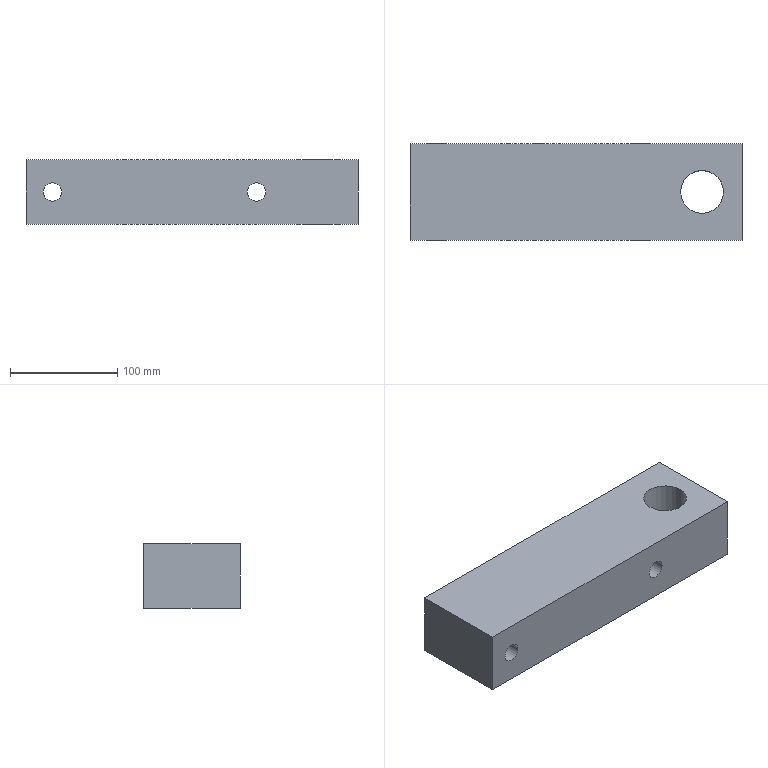Part | SolidWorks | features ICE 2, Extrusion 1, HoleWzd 1 | 1 solid | 16 faces | box 310 x 90 x 60 mm | volume 1555190 mm3 | cylinder 8 | plane 6 | cone 2 | commonest cylinder face diameters 17 x4 10.2 x2 40 x2
STEP:
#1=CARTESIAN_POINT('',(137.7,0.,60.));
#2=VERTEX_POINT('',#1);
#3=CARTESIAN_POINT('',(97.7,0.,60.));
#4=VERTEX_POINT('',#3);
#5=CARTESIAN_POINT('',(117.7,0.,60.));
#6=DIRECTION('',(0.,0.,-1.));
#7=DIRECTION('',(-1.,0.,0.));
#8=AXIS2_PLACEMENT_3D('',#5,#6,#7);
#9=CIRCLE('',#8,20.);
#10=EDGE_CURVE('',#2,#4,#9,.T.);
#11=ORIENTED_EDGE('',*,*,#10,.F.);
#12=CARTESIAN_POINT('',(137.7,0.,0.));
#13=VERTEX_POINT('',#12);
#14=CARTESIAN_POINT('',(137.7,0.,60.));
#15=DIRECTION('',(0.,0.,-1.));
#16=VECTOR('',#15,1000.);
#17=LINE('',#14,#16);
#18=EDGE_CURVE('',#2,#13,#17,.T.);
#19=ORIENTED_EDGE('',*,*,#18,.T.);
#20=CARTESIAN_POINT('',(97.7,0.,0.));
#21=VERTEX_POINT('',#20);
#22=CARTESIAN_POINT('',(117.7,0.,0.));
#23=DIRECTION('',(0.,0.,-1.));
#24=DIRECTION('',(-1.,0.,0.));
#25=AXIS2_PLACEMENT_3D('',#22,#23,#24);
#26=CIRCLE('',#25,20.);
#27=EDGE_CURVE('',#13,#21,#26,.T.);
#28=ORIENTED_EDGE('',*,*,#27,.T.);
#29=CARTESIAN_POINT('',(97.7,0.,60.));
#30=DIRECTION('',(0.,0.,-1.));
#31=VECTOR('',#30,1000.);
#32=LINE('',#29,#31);
#33=EDGE_CURVE('',#4,#21,#32,.T.);
#34=ORIENTED_EDGE('',*,*,#33,.F.);
#35=EDGE_LOOP('',(#11,#19,#28,#34));
#36=FACE_OUTER_BOUND('',#35,.T.);
#37=CARTESIAN_POINT('',(117.7,0.,60.));
#38=DIRECTION('',(0.,0.,-1.));
#39=DIRECTION('',(-1.,0.,0.));
#40=AXIS2_PLACEMENT_3D('',#37,#38,#39);
#41=CYLINDRICAL_SURFACE('',#40,20.);
#42=ADVANCED_FACE('',(#36),#41,.F.);
#43=CARTESIAN_POINT('',(-35.,14.75,24.9));
#44=VERTEX_POINT('',#43);
#45=CARTESIAN_POINT('',(-35.,14.75,35.1));
#46=VERTEX_POINT('',#45);
#47=CARTESIAN_POINT('',(-35.,14.75,30.));
#48=DIRECTION('',(0.,1.,0.));
#49=DIRECTION('',(0.,0.,1.));
#50=AXIS2_PLACEMENT_3D('',#47,#48,#49);
#51=CIRCLE('',#50,5.1);
#52=EDGE_CURVE('',#44,#46,#51,.T.);
#53=ORIENTED_EDGE('',*,*,#52,.F.);
#54=CARTESIAN_POINT('',(-35.,45.,24.9));
#55=VERTEX_POINT('',#54);
#56=CARTESIAN_POINT('',(-35.,45.,24.9));
#57=DIRECTION('',(0.,1.,0.));
#58=VECTOR('',#57,1000.);
#59=LINE('',#56,#58);
#60=EDGE_CURVE('',#44,#55,#59,.T.);
#61=ORIENTED_EDGE('',*,*,#60,.T.);
#62=CARTESIAN_POINT('',(-35.,45.,35.1));
#63=VERTEX_POINT('',#62);
#64=CARTESIAN_POINT('',(-35.,45.,30.));
#65=DIRECTION('',(0.,1.,0.));
#66=DIRECTION('',(0.,0.,1.));
#67=AXIS2_PLACEMENT_3D('',#64,#65,#66);
#68=CIRCLE('',#67,5.1);
#69=EDGE_CURVE('',#55,#63,#68,.T.);
#70=ORIENTED_EDGE('',*,*,#69,.T.);
#71=CARTESIAN_POINT('',(-35.,45.,35.1));
#72=DIRECTION('',(0.,1.,0.));
#73=VECTOR('',#72,1000.);
#74=LINE('',#71,#73);
#75=EDGE_CURVE('',#46,#63,#74,.T.);
#76=ORIENTED_EDGE('',*,*,#75,.F.);
#77=EDGE_LOOP('',(#53,#61,#70,#76));
#78=FACE_OUTER_BOUND('',#77,.T.);
#79=CARTESIAN_POINT('',(-35.,45.,30.));
#80=DIRECTION('',(0.,1.,0.));
#81=DIRECTION('',(0.,0.,1.));
#82=AXIS2_PLACEMENT_3D('',#79,#80,#81);
#83=CYLINDRICAL_SURFACE('',#82,5.1);
#84=ADVANCED_FACE('',(#78),#83,.F.);
#85=CARTESIAN_POINT('',(-35.,11.686,30.));
#86=VERTEX_POINT('',#85);
#87=CARTESIAN_POINT('',(-35.,14.75,35.1));
#88=DIRECTION('',(0.,0.515,0.8572));
#89=VECTOR('',#88,1000.);
#90=LINE('',#87,#89);
#91=EDGE_CURVE('',#86,#46,#90,.T.);
#92=ORIENTED_EDGE('',*,*,#91,.F.);
#93=CARTESIAN_POINT('',(-35.,14.75,24.9));
#94=DIRECTION('',(0.,0.515,-0.8572));
#95=VECTOR('',#94,1000.);
#96=LINE('',#93,#95);
#97=EDGE_CURVE('',#86,#44,#96,.T.);
#98=ORIENTED_EDGE('',*,*,#97,.T.);
#99=ORIENTED_EDGE('',*,*,#52,.T.);
#100=EDGE_LOOP('',(#92,#98,#99));
#101=FACE_OUTER_BOUND('',#100,.T.);
#102=CARTESIAN_POINT('',(-35.,14.75,30.));
#103=DIRECTION('',(0.,1.,0.));
#104=DIRECTION('',(0.,0.,1.));
#105=AXIS2_PLACEMENT_3D('',#102,#103,#104);
#106=CONICAL_SURFACE('',#105,5.1,1.03);
#107=ADVANCED_FACE('',(#101),#106,.F.);
#108=CARTESIAN_POINT('',(-121.75,-45.,30.));
#109=VERTEX_POINT('',#108);
#110=CARTESIAN_POINT('',(-138.75,-45.,30.));
#111=VERTEX_POINT('',#110);
#112=CARTESIAN_POINT('',(-130.25,-45.,30.));
#113=DIRECTION('',(0.,1.,0.));
#114=DIRECTION('',(-1.,0.,0.));
#115=AXIS2_PLACEMENT_3D('',#112,#113,#114);
#116=CIRCLE('',#115,8.5);
#117=EDGE_CURVE('',#109,#111,#116,.T.);
#118=ORIENTED_EDGE('',*,*,#117,.F.);
#119=CARTESIAN_POINT('',(-121.75,45.,30.));
#120=VERTEX_POINT('',#119);
#121=CARTESIAN_POINT('',(-121.75,-45.,30.));
#122=DIRECTION('',(0.,1.,0.));
#123=VECTOR('',#122,1000.);
#124=LINE('',#121,#123);
#125=EDGE_CURVE('',#109,#120,#124,.T.);
#126=ORIENTED_EDGE('',*,*,#125,.T.);
#127=CARTESIAN_POINT('',(-138.75,45.,30.));
#128=VERTEX_POINT('',#127);
#129=CARTESIAN_POINT('',(-130.25,45.,30.));
#130=DIRECTION('',(0.,1.,0.));
#131=DIRECTION('',(-1.,0.,0.));
#132=AXIS2_PLACEMENT_3D('',#129,#130,#131);
#133=CIRCLE('',#132,8.5);
#134=EDGE_CURVE('',#120,#128,#133,.T.);
#135=ORIENTED_EDGE('',*,*,#134,.T.);
#136=CARTESIAN_POINT('',(-138.75,-45.,30.));
#137=DIRECTION('',(0.,1.,0.));
#138=VECTOR('',#137,1000.);
#139=LINE('',#136,#138);
#140=EDGE_CURVE('',#111,#128,#139,.T.);
#141=ORIENTED_EDGE('',*,*,#140,.F.);
#142=EDGE_LOOP('',(#118,#126,#135,#141));
#143=FACE_OUTER_BOUND('',#142,.T.);
#144=CARTESIAN_POINT('',(-130.25,-45.,30.));
#145=DIRECTION('',(0.,1.,0.));
#146=DIRECTION('',(-1.,0.,0.));
#147=AXIS2_PLACEMENT_3D('',#144,#145,#146);
#148=CYLINDRICAL_SURFACE('',#147,8.5);
#149=ADVANCED_FACE('',(#143),#148,.F.);
#150=CARTESIAN_POINT('',(68.75,-45.,30.));
#151=VERTEX_POINT('',#150);
#152=CARTESIAN_POINT('',(51.75,-45.,30.));
#153=VERTEX_POINT('',#152);
#154=CARTESIAN_POINT('',(60.25,-45.,30.));
#155=DIRECTION('',(0.,1.,0.));
#156=DIRECTION('',(-1.,0.,0.));
#157=AXIS2_PLACEMENT_3D('',#154,#155,#156);
#158=CIRCLE('',#157,8.5);
#159=EDGE_CURVE('',#151,#153,#158,.T.);
#160=ORIENTED_EDGE('',*,*,#159,.F.);
#161=CARTESIAN_POINT('',(68.75,45.,30.));
#162=VERTEX_POINT('',#161);
#163=CARTESIAN_POINT('',(68.75,-45.,30.));
#164=DIRECTION('',(0.,1.,0.));
#165=VECTOR('',#164,1000.);
#166=LINE('',#163,#165);
#167=EDGE_CURVE('',#151,#162,#166,.T.);
#168=ORIENTED_EDGE('',*,*,#167,.T.);
#169=CARTESIAN_POINT('',(51.75,45.,30.));
#170=VERTEX_POINT('',#169);
#171=CARTESIAN_POINT('',(60.25,45.,30.));
#172=DIRECTION('',(0.,1.,0.));
#173=DIRECTION('',(-1.,0.,0.));
#174=AXIS2_PLACEMENT_3D('',#171,#172,#173);
#175=CIRCLE('',#174,8.5);
#176=EDGE_CURVE('',#162,#170,#175,.T.);
#177=ORIENTED_EDGE('',*,*,#176,.T.);
#178=CARTESIAN_POINT('',(51.75,-45.,30.));
#179=DIRECTION('',(0.,1.,0.));
#180=VECTOR('',#179,1000.);
#181=LINE('',#178,#180);
#182=EDGE_CURVE('',#153,#170,#181,.T.);
#183=ORIENTED_EDGE('',*,*,#182,.F.);
#184=EDGE_LOOP('',(#160,#168,#177,#183));
#185=FACE_OUTER_BOUND('',#184,.T.);
#186=CARTESIAN_POINT('',(60.25,-45.,30.));
#187=DIRECTION('',(0.,1.,0.));
#188=DIRECTION('',(-1.,0.,0.));
#189=AXIS2_PLACEMENT_3D('',#186,#187,#188);
#190=CYLINDRICAL_SURFACE('',#189,8.5);
#191=ADVANCED_FACE('',(#185),#190,.F.);
#192=CARTESIAN_POINT('',(-155.,45.,0.));
#193=VERTEX_POINT('',#192);
#194=CARTESIAN_POINT('',(-155.,-45.,0.));
#195=VERTEX_POINT('',#194);
#196=CARTESIAN_POINT('',(-155.,45.,0.));
#197=DIRECTION('',(0.,-1.,0.));
#198=VECTOR('',#197,1000.);
#199=LINE('',#196,#198);
#200=EDGE_CURVE('',#193,#195,#199,.T.);
#201=ORIENTED_EDGE('',*,*,#200,.T.);
#202=CARTESIAN_POINT('',(-155.,-45.,60.));
#203=VERTEX_POINT('',#202);
#204=CARTESIAN_POINT('',(-155.,-45.,60.));
#205=DIRECTION('',(0.,0.,-1.));
#206=VECTOR('',#205,1000.);
#207=LINE('',#204,#206);
#208=EDGE_CURVE('',#203,#195,#207,.T.);
#209=ORIENTED_EDGE('',*,*,#208,.F.);
#210=CARTESIAN_POINT('',(-155.,45.,60.));
#211=VERTEX_POINT('',#210);
#212=CARTESIAN_POINT('',(-155.,45.,60.));
#213=DIRECTION('',(0.,-1.,0.));
#214=VECTOR('',#213,1000.);
#215=LINE('',#212,#214);
#216=EDGE_CURVE('',#211,#203,#215,.T.);
#217=ORIENTED_EDGE('',*,*,#216,.F.);
#218=CARTESIAN_POINT('',(-155.,45.,60.));
#219=DIRECTION('',(0.,0.,-1.));
#220=VECTOR('',#219,1000.);
#221=LINE('',#218,#220);
#222=EDGE_CURVE('',#211,#193,#221,.T.);
#223=ORIENTED_EDGE('',*,*,#222,.T.);
#224=EDGE_LOOP('',(#201,#209,#217,#223));
#225=FACE_OUTER_BOUND('',#224,.T.);
#226=CARTESIAN_POINT('',(-155.,45.,60.));
#227=DIRECTION('',(1.,0.,0.));
#228=DIRECTION('',(0.,0.,-1.));
#229=AXIS2_PLACEMENT_3D('',#226,#227,#228);
#230=PLANE('',#229);
#231=ADVANCED_FACE('',(#225),#230,.F.);
#232=CARTESIAN_POINT('',(-130.25,-45.,30.));
#233=DIRECTION('',(0.,1.,0.));
#234=DIRECTION('',(-1.,0.,0.));
#235=AXIS2_PLACEMENT_3D('',#232,#233,#234);
#236=CIRCLE('',#235,8.5);
#237=EDGE_CURVE('',#111,#109,#236,.T.);
#238=ORIENTED_EDGE('',*,*,#237,.T.);
#239=ORIENTED_EDGE('',*,*,#117,.T.);
#240=EDGE_LOOP('',(#238,#239));
#241=FACE_BOUND('',#240,.T.);
#242=CARTESIAN_POINT('',(60.25,-45.,30.));
#243=DIRECTION('',(0.,1.,0.));
#244=DIRECTION('',(-1.,0.,0.));
#245=AXIS2_PLACEMENT_3D('',#242,#243,#244);
#246=CIRCLE('',#245,8.5);
#247=EDGE_CURVE('',#153,#151,#246,.T.);
#248=ORIENTED_EDGE('',*,*,#247,.T.);
#249=ORIENTED_EDGE('',*,*,#159,.T.);
#250=EDGE_LOOP('',(#248,#249));
#251=FACE_BOUND('',#250,.T.);
#252=CARTESIAN_POINT('',(155.,-45.,0.));
#253=VERTEX_POINT('',#252);
#254=CARTESIAN_POINT('',(155.,-45.,0.));
#255=DIRECTION('',(1.,0.,0.));
#256=VECTOR('',#255,1000.);
#257=LINE('',#254,#256);
#258=EDGE_CURVE('',#195,#253,#257,.T.);
#259=ORIENTED_EDGE('',*,*,#258,.T.);
#260=CARTESIAN_POINT('',(155.,-45.,60.));
#261=VERTEX_POINT('',#260);
#262=CARTESIAN_POINT('',(155.,-45.,60.));
#263=DIRECTION('',(0.,0.,-1.));
#264=VECTOR('',#263,1000.);
#265=LINE('',#262,#264);
#266=EDGE_CURVE('',#261,#253,#265,.T.);
#267=ORIENTED_EDGE('',*,*,#266,.F.);
#268=CARTESIAN_POINT('',(155.,-45.,60.));
#269=DIRECTION('',(1.,0.,0.));
#270=VECTOR('',#269,1000.);
#271=LINE('',#268,#270);
#272=EDGE_CURVE('',#203,#261,#271,.T.);
#273=ORIENTED_EDGE('',*,*,#272,.F.);
#274=ORIENTED_EDGE('',*,*,#208,.T.);
#275=EDGE_LOOP('',(#259,#267,#273,#274));
#276=FACE_OUTER_BOUND('',#275,.T.);
#277=CARTESIAN_POINT('',(155.,-45.,60.));
#278=DIRECTION('',(0.,1.,0.));
#279=DIRECTION('',(-1.,0.,0.));
#280=AXIS2_PLACEMENT_3D('',#277,#278,#279);
#281=PLANE('',#280);
#282=ADVANCED_FACE('',(#241,#251,#276),#281,.F.);
#283=CARTESIAN_POINT('',(155.,45.,0.));
#284=VERTEX_POINT('',#283);
#285=CARTESIAN_POINT('',(155.,45.,0.));
#286=DIRECTION('',(0.,1.,0.));
#287=VECTOR('',#286,1000.);
#288=LINE('',#285,#287);
#289=EDGE_CURVE('',#253,#284,#288,.T.);
#290=ORIENTED_EDGE('',*,*,#289,.T.);
#291=CARTESIAN_POINT('',(155.,45.,60.));
#292=VERTEX_POINT('',#291);
#293=CARTESIAN_POINT('',(155.,45.,60.));
#294=DIRECTION('',(0.,0.,-1.));
#295=VECTOR('',#294,1000.);
#296=LINE('',#293,#295);
#297=EDGE_CURVE('',#292,#284,#296,.T.);
#298=ORIENTED_EDGE('',*,*,#297,.F.);
#299=CARTESIAN_POINT('',(155.,45.,60.));
#300=DIRECTION('',(0.,1.,0.));
#301=VECTOR('',#300,1000.);
#302=LINE('',#299,#301);
#303=EDGE_CURVE('',#261,#292,#302,.T.);
#304=ORIENTED_EDGE('',*,*,#303,.F.);
#305=ORIENTED_EDGE('',*,*,#266,.T.);
#306=EDGE_LOOP('',(#290,#298,#304,#305));
#307=FACE_OUTER_BOUND('',#306,.T.);
#308=CARTESIAN_POINT('',(155.,45.,60.));
#309=DIRECTION('',(-1.,0.,0.));
#310=DIRECTION('',(0.,0.,1.));
#311=AXIS2_PLACEMENT_3D('',#308,#309,#310);
#312=PLANE('',#311);
#313=ADVANCED_FACE('',(#307),#312,.F.);
#314=CARTESIAN_POINT('',(-35.,45.,30.));
#315=DIRECTION('',(0.,1.,0.));
#316=DIRECTION('',(0.,0.,1.));
#317=AXIS2_PLACEMENT_3D('',#314,#315,#316);
#318=CIRCLE('',#317,5.1);
#319=EDGE_CURVE('',#63,#55,#318,.T.);
#320=ORIENTED_EDGE('',*,*,#319,.F.);
#321=ORIENTED_EDGE('',*,*,#69,.F.);
#322=EDGE_LOOP('',(#320,#321));
#323=FACE_BOUND('',#322,.T.);
#324=CARTESIAN_POINT('',(-130.25,45.,30.));
#325=DIRECTION('',(0.,1.,0.));
#326=DIRECTION('',(-1.,0.,0.));
#327=AXIS2_PLACEMENT_3D('',#324,#325,#326);
#328=CIRCLE('',#327,8.5);
#329=EDGE_CURVE('',#128,#120,#328,.T.);
#330=ORIENTED_EDGE('',*,*,#329,.F.);
#331=ORIENTED_EDGE('',*,*,#134,.F.);
#332=EDGE_LOOP('',(#330,#331));
#333=FACE_BOUND('',#332,.T.);
#334=CARTESIAN_POINT('',(60.25,45.,30.));
#335=DIRECTION('',(0.,1.,0.));
#336=DIRECTION('',(-1.,0.,0.));
#337=AXIS2_PLACEMENT_3D('',#334,#335,#336);
#338=CIRCLE('',#337,8.5);
#339=EDGE_CURVE('',#170,#162,#338,.T.);
#340=ORIENTED_EDGE('',*,*,#339,.F.);
#341=ORIENTED_EDGE('',*,*,#176,.F.);
#342=EDGE_LOOP('',(#340,#341));
#343=FACE_BOUND('',#342,.T.);
#344=CARTESIAN_POINT('',(155.,45.,0.));
#345=DIRECTION('',(-1.,0.,0.));
#346=VECTOR('',#345,1000.);
#347=LINE('',#344,#346);
#348=EDGE_CURVE('',#284,#193,#347,.T.);
#349=ORIENTED_EDGE('',*,*,#348,.T.);
#350=ORIENTED_EDGE('',*,*,#222,.F.);
#351=CARTESIAN_POINT('',(155.,45.,60.));
#352=DIRECTION('',(-1.,0.,0.));
#353=VECTOR('',#352,1000.);
#354=LINE('',#351,#353);
#355=EDGE_CURVE('',#292,#211,#354,.T.);
#356=ORIENTED_EDGE('',*,*,#355,.F.);
#357=ORIENTED_EDGE('',*,*,#297,.T.);
#358=EDGE_LOOP('',(#349,#350,#356,#357));
#359=FACE_OUTER_BOUND('',#358,.T.);
#360=CARTESIAN_POINT('',(155.,45.,60.));
#361=DIRECTION('',(0.,-1.,0.));
#362=DIRECTION('',(1.,0.,0.));
#363=AXIS2_PLACEMENT_3D('',#360,#361,#362);
#364=PLANE('',#363);
#365=ADVANCED_FACE('',(#323,#333,#343,#359),#364,.F.);
#366=CARTESIAN_POINT('',(117.7,0.,60.));
#367=DIRECTION('',(0.,0.,-1.));
#368=DIRECTION('',(-1.,0.,0.));
#369=AXIS2_PLACEMENT_3D('',#366,#367,#368);
#370=CIRCLE('',#369,20.);
#371=EDGE_CURVE('',#4,#2,#370,.T.);
#372=ORIENTED_EDGE('',*,*,#371,.T.);
#373=ORIENTED_EDGE('',*,*,#10,.T.);
#374=EDGE_LOOP('',(#372,#373));
#375=FACE_BOUND('',#374,.T.);
#376=ORIENTED_EDGE('',*,*,#216,.T.);
#377=ORIENTED_EDGE('',*,*,#272,.T.);
#378=ORIENTED_EDGE('',*,*,#303,.T.);
#379=ORIENTED_EDGE('',*,*,#355,.T.);
#380=EDGE_LOOP('',(#376,#377,#378,#379));
#381=FACE_OUTER_BOUND('',#380,.T.);
#382=CARTESIAN_POINT('',(0.,0.,60.));
#383=DIRECTION('',(0.,0.,-1.));
#384=DIRECTION('',(-1.,0.,0.));
#385=AXIS2_PLACEMENT_3D('',#382,#383,#384);
#386=PLANE('',#385);
#387=ADVANCED_FACE('',(#375,#381),#386,.F.);
#388=CARTESIAN_POINT('',(117.7,0.,0.));
#389=DIRECTION('',(0.,0.,-1.));
#390=DIRECTION('',(-1.,0.,0.));
#391=AXIS2_PLACEMENT_3D('',#388,#389,#390);
#392=CIRCLE('',#391,20.);
#393=EDGE_CURVE('',#21,#13,#392,.T.);
#394=ORIENTED_EDGE('',*,*,#393,.F.);
#395=ORIENTED_EDGE('',*,*,#27,.F.);
#396=EDGE_LOOP('',(#394,#395));
#397=FACE_BOUND('',#396,.T.);
#398=ORIENTED_EDGE('',*,*,#200,.F.);
#399=ORIENTED_EDGE('',*,*,#348,.F.);
#400=ORIENTED_EDGE('',*,*,#289,.F.);
#401=ORIENTED_EDGE('',*,*,#258,.F.);
#402=EDGE_LOOP('',(#398,#399,#400,#401));
#403=FACE_OUTER_BOUND('',#402,.T.);
#404=CARTESIAN_POINT('',(0.,0.,0.));
#405=DIRECTION('',(0.,0.,-1.));
#406=DIRECTION('',(-1.,0.,0.));
#407=AXIS2_PLACEMENT_3D('',#404,#405,#406);
#408=PLANE('',#407);
#409=ADVANCED_FACE('',(#397,#403),#408,.T.);
#410=ORIENTED_EDGE('',*,*,#167,.F.);
#411=ORIENTED_EDGE('',*,*,#247,.F.);
#412=ORIENTED_EDGE('',*,*,#182,.T.);
#413=ORIENTED_EDGE('',*,*,#339,.T.);
#414=EDGE_LOOP('',(#410,#411,#412,#413));
#415=FACE_OUTER_BOUND('',#414,.T.);
#416=CARTESIAN_POINT('',(60.25,-45.,30.));
#417=DIRECTION('',(0.,1.,0.));
#418=DIRECTION('',(-1.,0.,0.));
#419=AXIS2_PLACEMENT_3D('',#416,#417,#418);
#420=CYLINDRICAL_SURFACE('',#419,8.5);
#421=ADVANCED_FACE('',(#415),#420,.F.);
#422=ORIENTED_EDGE('',*,*,#125,.F.);
#423=ORIENTED_EDGE('',*,*,#237,.F.);
#424=ORIENTED_EDGE('',*,*,#140,.T.);
#425=ORIENTED_EDGE('',*,*,#329,.T.);
#426=EDGE_LOOP('',(#422,#423,#424,#425));
#427=FACE_OUTER_BOUND('',#426,.T.);
#428=CARTESIAN_POINT('',(-130.25,-45.,30.));
#429=DIRECTION('',(0.,1.,0.));
#430=DIRECTION('',(-1.,0.,0.));
#431=AXIS2_PLACEMENT_3D('',#428,#429,#430);
#432=CYLINDRICAL_SURFACE('',#431,8.5);
#433=ADVANCED_FACE('',(#427),#432,.F.);
#434=ORIENTED_EDGE('',*,*,#97,.F.);
#435=ORIENTED_EDGE('',*,*,#91,.T.);
#436=CARTESIAN_POINT('',(-35.,14.75,30.));
#437=DIRECTION('',(0.,1.,0.));
#438=DIRECTION('',(0.,0.,1.));
#439=AXIS2_PLACEMENT_3D('',#436,#437,#438);
#440=CIRCLE('',#439,5.1);
#441=EDGE_CURVE('',#46,#44,#440,.T.);
#442=ORIENTED_EDGE('',*,*,#441,.T.);
#443=EDGE_LOOP('',(#434,#435,#442));
#444=FACE_OUTER_BOUND('',#443,.T.);
#445=CARTESIAN_POINT('',(-35.,14.75,30.));
#446=DIRECTION('',(0.,1.,0.));
#447=DIRECTION('',(0.,0.,1.));
#448=AXIS2_PLACEMENT_3D('',#445,#446,#447);
#449=CONICAL_SURFACE('',#448,5.1,1.03);
#450=ADVANCED_FACE('',(#444),#449,.F.);
#451=ORIENTED_EDGE('',*,*,#60,.F.);
#452=ORIENTED_EDGE('',*,*,#441,.F.);
#453=ORIENTED_EDGE('',*,*,#75,.T.);
#454=ORIENTED_EDGE('',*,*,#319,.T.);
#455=EDGE_LOOP('',(#451,#452,#453,#454));
#456=FACE_OUTER_BOUND('',#455,.T.);
#457=CARTESIAN_POINT('',(-35.,45.,30.));
#458=DIRECTION('',(0.,1.,0.));
#459=DIRECTION('',(0.,0.,1.));
#460=AXIS2_PLACEMENT_3D('',#457,#458,#459);
#461=CYLINDRICAL_SURFACE('',#460,5.1);
#462=ADVANCED_FACE('',(#456),#461,.F.);
#463=ORIENTED_EDGE('',*,*,#18,.F.);
#464=ORIENTED_EDGE('',*,*,#371,.F.);
#465=ORIENTED_EDGE('',*,*,#33,.T.);
#466=ORIENTED_EDGE('',*,*,#393,.T.);
#467=EDGE_LOOP('',(#463,#464,#465,#466));
#468=FACE_OUTER_BOUND('',#467,.T.);
#469=CARTESIAN_POINT('',(117.7,0.,60.));
#470=DIRECTION('',(0.,0.,-1.));
#471=DIRECTION('',(-1.,0.,0.));
#472=AXIS2_PLACEMENT_3D('',#469,#470,#471);
#473=CYLINDRICAL_SURFACE('',#472,20.);
#474=ADVANCED_FACE('',(#468),#473,.F.);
#475=CLOSED_SHELL('',(#42,#84,#107,#149,#191,#231,#282,#313,#365,#387,#409,#421,#433,#450,#462,#474));
#476=MANIFOLD_SOLID_BREP('',#475);
#477=CARTESIAN_POINT('',(0.,0.,0.));
#478=DIRECTION('',(0.,0.,1.));
#479=DIRECTION('',(1.,0.,0.));
#480=AXIS2_PLACEMENT_3D('',#477,#478,#479);
#481=(LENGTH_UNIT()NAMED_UNIT(*)SI_UNIT(.MILLI.,.METRE.));
#482=UNCERTAINTY_MEASURE_WITH_UNIT(LENGTH_MEASURE(0.00001),#481,'','');
#483=(NAMED_UNIT(*)PLANE_ANGLE_UNIT()SI_UNIT($,.RADIAN.));
#484=(NAMED_UNIT(*)SI_UNIT($,.STERADIAN.)SOLID_ANGLE_UNIT());
#485=(GEOMETRIC_REPRESENTATION_CONTEXT(3)GLOBAL_UNCERTAINTY_ASSIGNED_CONTEXT((#482))GLOBAL_UNIT_ASSIGNED_CONTEXT((#481,#483,#484))REPRESENTATION_CONTEXT('',''));
#486=ADVANCED_BREP_SHAPE_REPRESENTATION('',(#476,#480),#485);